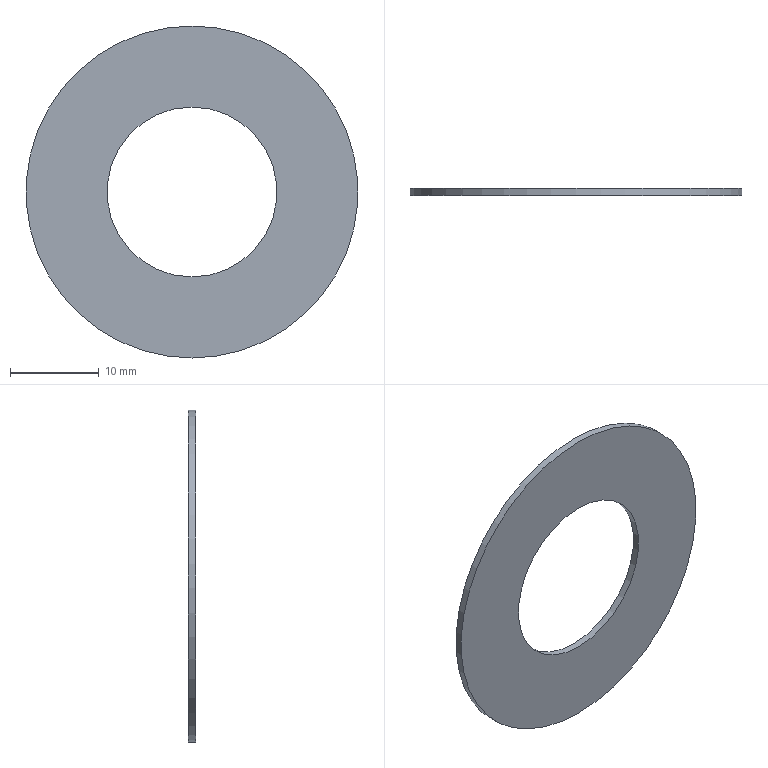Part | NX | features MG0330 trunion parts 24(trunion group) 2 | 1 solid | 4 faces | box 37.465 x 0.8128 x 37.465 mm | volume 661.269 mm3 | cylinder 2 | plane 2 | commonest cylinder face diameters 19.177 x1 37.465 x1
STEP:
#1=CARTESIAN_POINT('',(0.,16.65,-9.588));
#2=VERTEX_POINT('',#1);
#3=CARTESIAN_POINT('',(0.,16.65,0.));
#4=DIRECTION('',(0.,-1.,0.));
#5=DIRECTION('',(0.,0.,-1.));
#6=AXIS2_PLACEMENT_3D('',#3,#4,#5);
#7=CIRCLE('',#6,9.588);
#8=EDGE_CURVE('',#2,#2,#7,.T.);
#9=ORIENTED_EDGE('',*,*,#8,.T.);
#10=EDGE_LOOP('',(#9));
#11=FACE_BOUND('',#10,.T.);
#12=CARTESIAN_POINT('',(0.,17.462,-9.588));
#13=VERTEX_POINT('',#12);
#14=CARTESIAN_POINT('',(0.,17.462,0.));
#15=DIRECTION('',(0.,-1.,0.));
#16=DIRECTION('',(0.,0.,-1.));
#17=AXIS2_PLACEMENT_3D('',#14,#15,#16);
#18=CIRCLE('',#17,9.588);
#19=EDGE_CURVE('',#13,#13,#18,.T.);
#20=ORIENTED_EDGE('',*,*,#19,.F.);
#21=EDGE_LOOP('',(#20));
#22=FACE_BOUND('',#21,.T.);
#23=CARTESIAN_POINT('',(0.,0.,0.));
#24=DIRECTION('',(0.,-1.,0.));
#25=DIRECTION('',(0.,0.,-1.));
#26=AXIS2_PLACEMENT_3D('',#23,#24,#25);
#27=CYLINDRICAL_SURFACE('',#26,9.588);
#28=ADVANCED_FACE('',(#11,#22),#27,.F.);
#29=CARTESIAN_POINT('',(0.,16.65,-18.733));
#30=VERTEX_POINT('',#29);
#31=CARTESIAN_POINT('',(0.,16.65,0.));
#32=DIRECTION('',(0.,-1.,0.));
#33=DIRECTION('',(0.,0.,-1.));
#34=AXIS2_PLACEMENT_3D('',#31,#32,#33);
#35=CIRCLE('',#34,18.733);
#36=EDGE_CURVE('',#30,#30,#35,.T.);
#37=ORIENTED_EDGE('',*,*,#36,.T.);
#38=EDGE_LOOP('',(#37));
#39=FACE_BOUND('',#38,.T.);
#40=ORIENTED_EDGE('',*,*,#8,.F.);
#41=EDGE_LOOP('',(#40));
#42=FACE_BOUND('',#41,.T.);
#43=CARTESIAN_POINT('',(9.588,16.65,0.));
#44=DIRECTION('',(0.,-1.,0.));
#45=DIRECTION('',(0.,0.,-1.));
#46=AXIS2_PLACEMENT_3D('',#43,#44,#45);
#47=PLANE('',#46);
#48=ADVANCED_FACE('',(#39,#42),#47,.T.);
#49=CARTESIAN_POINT('',(0.,17.462,-18.733));
#50=VERTEX_POINT('',#49);
#51=CARTESIAN_POINT('',(0.,17.462,0.));
#52=DIRECTION('',(0.,-1.,0.));
#53=DIRECTION('',(0.,0.,-1.));
#54=AXIS2_PLACEMENT_3D('',#51,#52,#53);
#55=CIRCLE('',#54,18.733);
#56=EDGE_CURVE('',#50,#50,#55,.T.);
#57=ORIENTED_EDGE('',*,*,#56,.T.);
#58=EDGE_LOOP('',(#57));
#59=FACE_BOUND('',#58,.T.);
#60=ORIENTED_EDGE('',*,*,#36,.F.);
#61=EDGE_LOOP('',(#60));
#62=FACE_BOUND('',#61,.T.);
#63=CARTESIAN_POINT('',(0.,0.,0.));
#64=DIRECTION('',(0.,-1.,0.));
#65=DIRECTION('',(0.,0.,-1.));
#66=AXIS2_PLACEMENT_3D('',#63,#64,#65);
#67=CYLINDRICAL_SURFACE('',#66,18.733);
#68=ADVANCED_FACE('',(#59,#62),#67,.T.);
#69=ORIENTED_EDGE('',*,*,#19,.T.);
#70=EDGE_LOOP('',(#69));
#71=FACE_BOUND('',#70,.T.);
#72=ORIENTED_EDGE('',*,*,#56,.F.);
#73=EDGE_LOOP('',(#72));
#74=FACE_BOUND('',#73,.T.);
#75=CARTESIAN_POINT('',(9.588,17.462,0.));
#76=DIRECTION('',(0.,1.,0.));
#77=DIRECTION('',(0.,0.,1.));
#78=AXIS2_PLACEMENT_3D('',#75,#76,#77);
#79=PLANE('',#78);
#80=ADVANCED_FACE('',(#71,#74),#79,.T.);
#81=CLOSED_SHELL('',(#28,#48,#68,#80));
#82=MANIFOLD_SOLID_BREP('',#81);
#83=(LENGTH_UNIT()NAMED_UNIT(*)SI_UNIT(.MILLI.,.METRE.));
#84=UNCERTAINTY_MEASURE_WITH_UNIT(LENGTH_MEASURE(0.00001),#83,'','');
#85=(NAMED_UNIT(*)PLANE_ANGLE_UNIT()SI_UNIT($,.RADIAN.));
#86=(NAMED_UNIT(*)SI_UNIT($,.STERADIAN.)SOLID_ANGLE_UNIT());
#87=(GEOMETRIC_REPRESENTATION_CONTEXT(3)GLOBAL_UNCERTAINTY_ASSIGNED_CONTEXT((#84))GLOBAL_UNIT_ASSIGNED_CONTEXT((#83,#85,#86))REPRESENTATION_CONTEXT('',''));
#88=ADVANCED_BREP_SHAPE_REPRESENTATION('',(#82),#87);